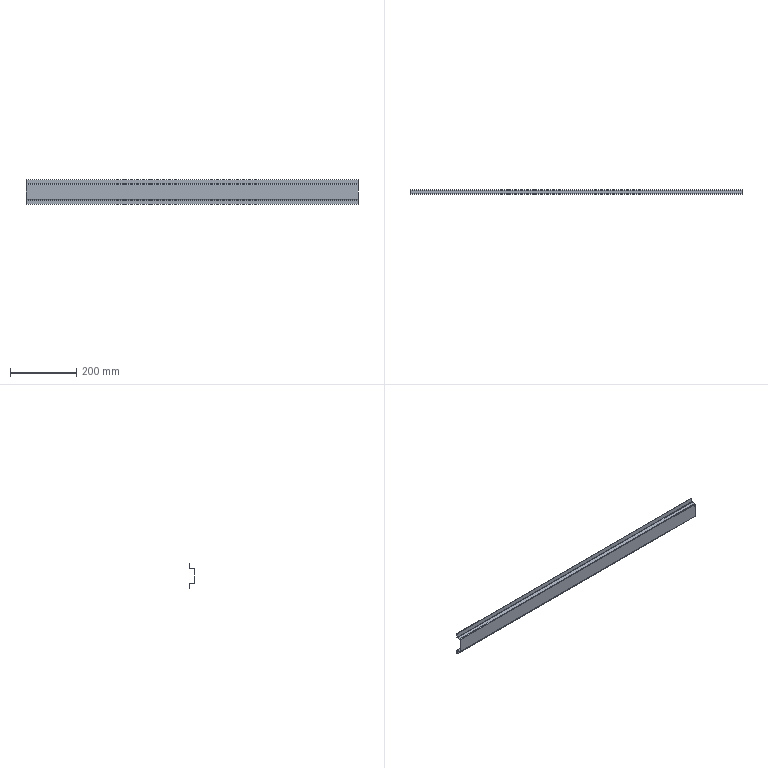Part | SolidWorks | features BaseBody 1 | 1 solid | 22 faces | box 1005 x 14.5 x 75 mm | volume 100376 mm3 | plane 14 | cylinder 8 | commonest cylinder face diameters 1.473 x4 3.473 x4
STEP:
#1=CARTESIAN_POINT('',(502.5,0.,21.763));
#2=VERTEX_POINT('',#1);
#3=CARTESIAN_POINT('',(-502.5,0.,21.763));
#4=VERTEX_POINT('',#3);
#5=CARTESIAN_POINT('',(502.5,0.,21.763));
#6=DIRECTION('',(-1.,0.,0.));
#7=VECTOR('',#6,1000.);
#8=LINE('',#5,#7);
#9=EDGE_CURVE('',#2,#4,#8,.T.);
#10=ORIENTED_EDGE('',*,*,#9,.F.);
#11=CARTESIAN_POINT('',(502.5,0.,-21.763));
#12=VERTEX_POINT('',#11);
#13=CARTESIAN_POINT('',(502.5,0.,22.5));
#14=DIRECTION('',(0.,0.,1.));
#15=VECTOR('',#14,1000.);
#16=LINE('',#13,#15);
#17=EDGE_CURVE('',#12,#2,#16,.T.);
#18=ORIENTED_EDGE('',*,*,#17,.F.);
#19=CARTESIAN_POINT('',(-502.5,0.,-21.763));
#20=VERTEX_POINT('',#19);
#21=CARTESIAN_POINT('',(502.5,0.,-21.763));
#22=DIRECTION('',(1.,0.,0.));
#23=VECTOR('',#22,1000.);
#24=LINE('',#21,#23);
#25=EDGE_CURVE('',#20,#12,#24,.T.);
#26=ORIENTED_EDGE('',*,*,#25,.F.);
#27=CARTESIAN_POINT('',(-502.5,0.,22.5));
#28=DIRECTION('',(0.,0.,-1.));
#29=VECTOR('',#28,1000.);
#30=LINE('',#27,#29);
#31=EDGE_CURVE('',#4,#20,#30,.T.);
#32=ORIENTED_EDGE('',*,*,#31,.F.);
#33=EDGE_LOOP('',(#10,#18,#26,#32));
#34=FACE_OUTER_BOUND('',#33,.T.);
#35=CARTESIAN_POINT('',(502.5,0.,22.5));
#36=DIRECTION('',(0.,-1.,0.));
#37=DIRECTION('',(0.,0.,-1.));
#38=AXIS2_PLACEMENT_3D('',#35,#36,#37);
#39=PLANE('',#38);
#40=ADVANCED_FACE('',(#34),#39,.F.);
#41=CARTESIAN_POINT('',(-502.5,-1.,-21.763));
#42=VERTEX_POINT('',#41);
#43=CARTESIAN_POINT('',(-502.5,-1.,21.763));
#44=VERTEX_POINT('',#43);
#45=CARTESIAN_POINT('',(-502.5,-1.,-23.5));
#46=DIRECTION('',(0.,0.,1.));
#47=VECTOR('',#46,1000.);
#48=LINE('',#45,#47);
#49=EDGE_CURVE('',#42,#44,#48,.T.);
#50=ORIENTED_EDGE('',*,*,#49,.T.);
#51=CARTESIAN_POINT('',(-502.5,0.7366,23.5));
#52=VERTEX_POINT('',#51);
#53=CARTESIAN_POINT('',(-502.5,0.7366,21.763));
#54=DIRECTION('',(1.,0.,0.));
#55=DIRECTION('',(0.,0.,1.));
#56=AXIS2_PLACEMENT_3D('',#53,#54,#55);
#57=CIRCLE('',#56,1.737);
#58=EDGE_CURVE('',#52,#44,#57,.T.);
#59=ORIENTED_EDGE('',*,*,#58,.F.);
#60=CARTESIAN_POINT('',(-502.5,11.763,23.5));
#61=VERTEX_POINT('',#60);
#62=CARTESIAN_POINT('',(-502.5,-1.,23.5));
#63=DIRECTION('',(0.,1.,0.));
#64=VECTOR('',#63,1000.);
#65=LINE('',#62,#64);
#66=EDGE_CURVE('',#52,#61,#65,.T.);
#67=ORIENTED_EDGE('',*,*,#66,.T.);
#68=CARTESIAN_POINT('',(-502.5,12.5,24.237));
#69=VERTEX_POINT('',#68);
#70=CARTESIAN_POINT('',(-502.5,11.763,24.237));
#71=DIRECTION('',(1.,0.,0.));
#72=DIRECTION('',(0.,0.,1.));
#73=AXIS2_PLACEMENT_3D('',#70,#71,#72);
#74=CIRCLE('',#73,0.7366);
#75=EDGE_CURVE('',#61,#69,#74,.T.);
#76=ORIENTED_EDGE('',*,*,#75,.T.);
#77=CARTESIAN_POINT('',(-502.5,12.5,37.5));
#78=VERTEX_POINT('',#77);
#79=CARTESIAN_POINT('',(-502.5,12.5,23.5));
#80=DIRECTION('',(0.,0.,1.));
#81=VECTOR('',#80,1000.);
#82=LINE('',#79,#81);
#83=EDGE_CURVE('',#69,#78,#82,.T.);
#84=ORIENTED_EDGE('',*,*,#83,.T.);
#85=CARTESIAN_POINT('',(-502.5,13.5,37.5));
#86=VERTEX_POINT('',#85);
#87=CARTESIAN_POINT('',(-502.5,11.763,37.5));
#88=DIRECTION('',(0.,1.,0.));
#89=VECTOR('',#88,1000.);
#90=LINE('',#87,#89);
#91=EDGE_CURVE('',#78,#86,#90,.T.);
#92=ORIENTED_EDGE('',*,*,#91,.T.);
#93=CARTESIAN_POINT('',(-502.5,13.5,24.237));
#94=VERTEX_POINT('',#93);
#95=CARTESIAN_POINT('',(-502.5,13.5,22.5));
#96=DIRECTION('',(0.,0.,-1.));
#97=VECTOR('',#96,1000.);
#98=LINE('',#95,#97);
#99=EDGE_CURVE('',#86,#94,#98,.T.);
#100=ORIENTED_EDGE('',*,*,#99,.T.);
#101=CARTESIAN_POINT('',(-502.5,11.763,22.5));
#102=VERTEX_POINT('',#101);
#103=CARTESIAN_POINT('',(-502.5,11.763,24.237));
#104=DIRECTION('',(1.,0.,0.));
#105=DIRECTION('',(0.,0.,1.));
#106=AXIS2_PLACEMENT_3D('',#103,#104,#105);
#107=CIRCLE('',#106,1.737);
#108=EDGE_CURVE('',#102,#94,#107,.T.);
#109=ORIENTED_EDGE('',*,*,#108,.F.);
#110=CARTESIAN_POINT('',(-502.5,0.7366,22.5));
#111=VERTEX_POINT('',#110);
#112=CARTESIAN_POINT('',(-502.5,0.,22.5));
#113=DIRECTION('',(0.,-1.,0.));
#114=VECTOR('',#113,1000.);
#115=LINE('',#112,#114);
#116=EDGE_CURVE('',#102,#111,#115,.T.);
#117=ORIENTED_EDGE('',*,*,#116,.T.);
#118=CARTESIAN_POINT('',(-502.5,0.7366,21.763));
#119=DIRECTION('',(1.,0.,0.));
#120=DIRECTION('',(0.,0.,1.));
#121=AXIS2_PLACEMENT_3D('',#118,#119,#120);
#122=CIRCLE('',#121,0.7366);
#123=EDGE_CURVE('',#111,#4,#122,.T.);
#124=ORIENTED_EDGE('',*,*,#123,.T.);
#125=ORIENTED_EDGE('',*,*,#31,.T.);
#126=CARTESIAN_POINT('',(-502.5,0.7366,-22.5));
#127=VERTEX_POINT('',#126);
#128=CARTESIAN_POINT('',(-502.5,0.7366,-21.763));
#129=DIRECTION('',(1.,0.,0.));
#130=DIRECTION('',(0.,0.,1.));
#131=AXIS2_PLACEMENT_3D('',#128,#129,#130);
#132=CIRCLE('',#131,0.7366);
#133=EDGE_CURVE('',#20,#127,#132,.T.);
#134=ORIENTED_EDGE('',*,*,#133,.T.);
#135=CARTESIAN_POINT('',(-502.5,11.763,-22.5));
#136=VERTEX_POINT('',#135);
#137=CARTESIAN_POINT('',(-502.5,0.,-22.5));
#138=DIRECTION('',(0.,1.,0.));
#139=VECTOR('',#138,1000.);
#140=LINE('',#137,#139);
#141=EDGE_CURVE('',#127,#136,#140,.T.);
#142=ORIENTED_EDGE('',*,*,#141,.T.);
#143=CARTESIAN_POINT('',(-502.5,13.5,-24.237));
#144=VERTEX_POINT('',#143);
#145=CARTESIAN_POINT('',(-502.5,11.763,-24.237));
#146=DIRECTION('',(1.,0.,0.));
#147=DIRECTION('',(0.,0.,1.));
#148=AXIS2_PLACEMENT_3D('',#145,#146,#147);
#149=CIRCLE('',#148,1.737);
#150=EDGE_CURVE('',#144,#136,#149,.T.);
#151=ORIENTED_EDGE('',*,*,#150,.F.);
#152=CARTESIAN_POINT('',(-502.5,13.5,-37.5));
#153=VERTEX_POINT('',#152);
#154=CARTESIAN_POINT('',(-502.5,13.5,-22.5));
#155=DIRECTION('',(0.,0.,-1.));
#156=VECTOR('',#155,1000.);
#157=LINE('',#154,#156);
#158=EDGE_CURVE('',#144,#153,#157,.T.);
#159=ORIENTED_EDGE('',*,*,#158,.T.);
#160=CARTESIAN_POINT('',(-502.5,12.5,-37.5));
#161=VERTEX_POINT('',#160);
#162=CARTESIAN_POINT('',(-502.5,11.763,-37.5));
#163=DIRECTION('',(0.,1.,0.));
#164=VECTOR('',#163,1000.);
#165=LINE('',#162,#164);
#166=EDGE_CURVE('',#161,#153,#165,.T.);
#167=ORIENTED_EDGE('',*,*,#166,.F.);
#168=CARTESIAN_POINT('',(-502.5,12.5,-24.237));
#169=VERTEX_POINT('',#168);
#170=CARTESIAN_POINT('',(-502.5,12.5,24.237));
#171=DIRECTION('',(0.,0.,-1.));
#172=VECTOR('',#171,1000.);
#173=LINE('',#170,#172);
#174=EDGE_CURVE('',#169,#161,#173,.T.);
#175=ORIENTED_EDGE('',*,*,#174,.F.);
#176=CARTESIAN_POINT('',(-502.5,11.763,-23.5));
#177=VERTEX_POINT('',#176);
#178=CARTESIAN_POINT('',(-502.5,11.763,-24.237));
#179=DIRECTION('',(1.,0.,0.));
#180=DIRECTION('',(0.,0.,1.));
#181=AXIS2_PLACEMENT_3D('',#178,#179,#180);
#182=CIRCLE('',#181,0.7366);
#183=EDGE_CURVE('',#169,#177,#182,.T.);
#184=ORIENTED_EDGE('',*,*,#183,.T.);
#185=CARTESIAN_POINT('',(-502.5,0.7366,-23.5));
#186=VERTEX_POINT('',#185);
#187=CARTESIAN_POINT('',(-502.5,12.5,-23.5));
#188=DIRECTION('',(0.,-1.,0.));
#189=VECTOR('',#188,1000.);
#190=LINE('',#187,#189);
#191=EDGE_CURVE('',#177,#186,#190,.T.);
#192=ORIENTED_EDGE('',*,*,#191,.T.);
#193=CARTESIAN_POINT('',(-502.5,0.7366,-21.763));
#194=DIRECTION('',(1.,0.,0.));
#195=DIRECTION('',(0.,0.,1.));
#196=AXIS2_PLACEMENT_3D('',#193,#194,#195);
#197=CIRCLE('',#196,1.737);
#198=EDGE_CURVE('',#42,#186,#197,.T.);
#199=ORIENTED_EDGE('',*,*,#198,.F.);
#200=EDGE_LOOP('',(#50,#59,#67,#76,#84,#92,#100,#109,#117,#124,#125,#134,#142,#151,#159,#167,#175,#184,#192,#199));
#201=FACE_OUTER_BOUND('',#200,.T.);
#202=CARTESIAN_POINT('',(-502.5,0.7366,-23.5));
#203=DIRECTION('',(-1.,0.,0.));
#204=DIRECTION('',(0.,0.,1.));
#205=AXIS2_PLACEMENT_3D('',#202,#203,#204);
#206=PLANE('',#205);
#207=ADVANCED_FACE('',(#201),#206,.T.);
#208=CARTESIAN_POINT('',(502.5,0.7366,22.5));
#209=VERTEX_POINT('',#208);
#210=CARTESIAN_POINT('',(502.5,0.7366,22.5));
#211=DIRECTION('',(-1.,0.,0.));
#212=VECTOR('',#211,1000.);
#213=LINE('',#210,#212);
#214=EDGE_CURVE('',#209,#111,#213,.T.);
#215=ORIENTED_EDGE('',*,*,#214,.F.);
#216=CARTESIAN_POINT('',(502.5,0.7366,21.763));
#217=DIRECTION('',(-1.,0.,0.));
#218=DIRECTION('',(0.,0.,1.));
#219=AXIS2_PLACEMENT_3D('',#216,#217,#218);
#220=CIRCLE('',#219,0.7366);
#221=EDGE_CURVE('',#2,#209,#220,.T.);
#222=ORIENTED_EDGE('',*,*,#221,.F.);
#223=ORIENTED_EDGE('',*,*,#9,.T.);
#224=ORIENTED_EDGE('',*,*,#123,.F.);
#225=EDGE_LOOP('',(#215,#222,#223,#224));
#226=FACE_OUTER_BOUND('',#225,.T.);
#227=CARTESIAN_POINT('',(502.5,0.7366,21.763));
#228=DIRECTION('',(-1.,0.,0.));
#229=DIRECTION('',(0.,0.,1.));
#230=AXIS2_PLACEMENT_3D('',#227,#228,#229);
#231=CYLINDRICAL_SURFACE('',#230,0.7366);
#232=ADVANCED_FACE('',(#226),#231,.F.);
#233=CARTESIAN_POINT('',(502.5,-1.,21.763));
#234=VERTEX_POINT('',#233);
#235=CARTESIAN_POINT('',(502.5,-1.,-21.763));
#236=VERTEX_POINT('',#235);
#237=CARTESIAN_POINT('',(502.5,-1.,23.5));
#238=DIRECTION('',(0.,0.,-1.));
#239=VECTOR('',#238,1000.);
#240=LINE('',#237,#239);
#241=EDGE_CURVE('',#234,#236,#240,.T.);
#242=ORIENTED_EDGE('',*,*,#241,.T.);
#243=CARTESIAN_POINT('',(502.5,0.7366,-23.5));
#244=VERTEX_POINT('',#243);
#245=CARTESIAN_POINT('',(502.5,0.7366,-21.763));
#246=DIRECTION('',(-1.,0.,0.));
#247=DIRECTION('',(0.,0.,1.));
#248=AXIS2_PLACEMENT_3D('',#245,#246,#247);
#249=CIRCLE('',#248,1.737);
#250=EDGE_CURVE('',#244,#236,#249,.T.);
#251=ORIENTED_EDGE('',*,*,#250,.F.);
#252=CARTESIAN_POINT('',(502.5,11.763,-23.5));
#253=VERTEX_POINT('',#252);
#254=CARTESIAN_POINT('',(502.5,-1.,-23.5));
#255=DIRECTION('',(0.,1.,0.));
#256=VECTOR('',#255,1000.);
#257=LINE('',#254,#256);
#258=EDGE_CURVE('',#244,#253,#257,.T.);
#259=ORIENTED_EDGE('',*,*,#258,.T.);
#260=CARTESIAN_POINT('',(502.5,12.5,-24.237));
#261=VERTEX_POINT('',#260);
#262=CARTESIAN_POINT('',(502.5,11.763,-24.237));
#263=DIRECTION('',(-1.,0.,0.));
#264=DIRECTION('',(0.,0.,1.));
#265=AXIS2_PLACEMENT_3D('',#262,#263,#264);
#266=CIRCLE('',#265,0.7366);
#267=EDGE_CURVE('',#253,#261,#266,.T.);
#268=ORIENTED_EDGE('',*,*,#267,.T.);
#269=CARTESIAN_POINT('',(502.5,12.5,-37.5));
#270=VERTEX_POINT('',#269);
#271=CARTESIAN_POINT('',(502.5,12.5,-23.5));
#272=DIRECTION('',(0.,0.,-1.));
#273=VECTOR('',#272,1000.);
#274=LINE('',#271,#273);
#275=EDGE_CURVE('',#261,#270,#274,.T.);
#276=ORIENTED_EDGE('',*,*,#275,.T.);
#277=CARTESIAN_POINT('',(502.5,13.5,-37.5));
#278=VERTEX_POINT('',#277);
#279=CARTESIAN_POINT('',(502.5,11.763,-37.5));
#280=DIRECTION('',(0.,1.,0.));
#281=VECTOR('',#280,1000.);
#282=LINE('',#279,#281);
#283=EDGE_CURVE('',#270,#278,#282,.T.);
#284=ORIENTED_EDGE('',*,*,#283,.T.);
#285=CARTESIAN_POINT('',(502.5,13.5,-24.237));
#286=VERTEX_POINT('',#285);
#287=CARTESIAN_POINT('',(502.5,13.5,-22.5));
#288=DIRECTION('',(0.,0.,1.));
#289=VECTOR('',#288,1000.);
#290=LINE('',#287,#289);
#291=EDGE_CURVE('',#278,#286,#290,.T.);
#292=ORIENTED_EDGE('',*,*,#291,.T.);
#293=CARTESIAN_POINT('',(502.5,11.763,-22.5));
#294=VERTEX_POINT('',#293);
#295=CARTESIAN_POINT('',(502.5,11.763,-24.237));
#296=DIRECTION('',(-1.,0.,0.));
#297=DIRECTION('',(0.,0.,1.));
#298=AXIS2_PLACEMENT_3D('',#295,#296,#297);
#299=CIRCLE('',#298,1.737);
#300=EDGE_CURVE('',#294,#286,#299,.T.);
#301=ORIENTED_EDGE('',*,*,#300,.F.);
#302=CARTESIAN_POINT('',(502.5,0.7366,-22.5));
#303=VERTEX_POINT('',#302);
#304=CARTESIAN_POINT('',(502.5,0.,-22.5));
#305=DIRECTION('',(0.,-1.,0.));
#306=VECTOR('',#305,1000.);
#307=LINE('',#304,#306);
#308=EDGE_CURVE('',#294,#303,#307,.T.);
#309=ORIENTED_EDGE('',*,*,#308,.T.);
#310=CARTESIAN_POINT('',(502.5,0.7366,-21.763));
#311=DIRECTION('',(-1.,0.,0.));
#312=DIRECTION('',(0.,0.,1.));
#313=AXIS2_PLACEMENT_3D('',#310,#311,#312);
#314=CIRCLE('',#313,0.7366);
#315=EDGE_CURVE('',#303,#12,#314,.T.);
#316=ORIENTED_EDGE('',*,*,#315,.T.);
#317=ORIENTED_EDGE('',*,*,#17,.T.);
#318=ORIENTED_EDGE('',*,*,#221,.T.);
#319=CARTESIAN_POINT('',(502.5,11.763,22.5));
#320=VERTEX_POINT('',#319);
#321=CARTESIAN_POINT('',(502.5,0.,22.5));
#322=DIRECTION('',(0.,1.,0.));
#323=VECTOR('',#322,1000.);
#324=LINE('',#321,#323);
#325=EDGE_CURVE('',#209,#320,#324,.T.);
#326=ORIENTED_EDGE('',*,*,#325,.T.);
#327=CARTESIAN_POINT('',(502.5,13.5,24.237));
#328=VERTEX_POINT('',#327);
#329=CARTESIAN_POINT('',(502.5,11.763,24.237));
#330=DIRECTION('',(-1.,0.,0.));
#331=DIRECTION('',(0.,0.,1.));
#332=AXIS2_PLACEMENT_3D('',#329,#330,#331);
#333=CIRCLE('',#332,1.737);
#334=EDGE_CURVE('',#328,#320,#333,.T.);
#335=ORIENTED_EDGE('',*,*,#334,.F.);
#336=CARTESIAN_POINT('',(502.5,13.5,37.5));
#337=VERTEX_POINT('',#336);
#338=CARTESIAN_POINT('',(502.5,13.5,22.5));
#339=DIRECTION('',(0.,0.,1.));
#340=VECTOR('',#339,1000.);
#341=LINE('',#338,#340);
#342=EDGE_CURVE('',#328,#337,#341,.T.);
#343=ORIENTED_EDGE('',*,*,#342,.T.);
#344=CARTESIAN_POINT('',(502.5,12.5,37.5));
#345=VERTEX_POINT('',#344);
#346=CARTESIAN_POINT('',(502.5,12.5,37.5));
#347=DIRECTION('',(0.,1.,0.));
#348=VECTOR('',#347,1000.);
#349=LINE('',#346,#348);
#350=EDGE_CURVE('',#345,#337,#349,.T.);
#351=ORIENTED_EDGE('',*,*,#350,.F.);
#352=CARTESIAN_POINT('',(502.5,12.5,24.237));
#353=VERTEX_POINT('',#352);
#354=CARTESIAN_POINT('',(502.5,12.5,24.237));
#355=DIRECTION('',(0.,0.,-1.));
#356=VECTOR('',#355,1000.);
#357=LINE('',#354,#356);
#358=EDGE_CURVE('',#345,#353,#357,.T.);
#359=ORIENTED_EDGE('',*,*,#358,.T.);
#360=CARTESIAN_POINT('',(502.5,11.763,23.5));
#361=VERTEX_POINT('',#360);
#362=CARTESIAN_POINT('',(502.5,11.763,24.237));
#363=DIRECTION('',(-1.,0.,0.));
#364=DIRECTION('',(0.,0.,1.));
#365=AXIS2_PLACEMENT_3D('',#362,#363,#364);
#366=CIRCLE('',#365,0.7366);
#367=EDGE_CURVE('',#353,#361,#366,.T.);
#368=ORIENTED_EDGE('',*,*,#367,.T.);
#369=CARTESIAN_POINT('',(502.5,0.7366,23.5));
#370=VERTEX_POINT('',#369);
#371=CARTESIAN_POINT('',(502.5,12.5,23.5));
#372=DIRECTION('',(0.,-1.,0.));
#373=VECTOR('',#372,1000.);
#374=LINE('',#371,#373);
#375=EDGE_CURVE('',#361,#370,#374,.T.);
#376=ORIENTED_EDGE('',*,*,#375,.T.);
#377=CARTESIAN_POINT('',(502.5,0.7366,21.763));
#378=DIRECTION('',(-1.,0.,0.));
#379=DIRECTION('',(0.,0.,1.));
#380=AXIS2_PLACEMENT_3D('',#377,#378,#379);
#381=CIRCLE('',#380,1.737);
#382=EDGE_CURVE('',#234,#370,#381,.T.);
#383=ORIENTED_EDGE('',*,*,#382,.F.);
#384=EDGE_LOOP('',(#242,#251,#259,#268,#276,#284,#292,#301,#309,#316,#317,#318,#326,#335,#343,#351,#359,#368,#376,#383));
#385=FACE_OUTER_BOUND('',#384,.T.);
#386=CARTESIAN_POINT('',(502.5,0.7366,23.5));
#387=DIRECTION('',(1.,0.,0.));
#388=DIRECTION('',(0.,0.,-1.));
#389=AXIS2_PLACEMENT_3D('',#386,#387,#388);
#390=PLANE('',#389);
#391=ADVANCED_FACE('',(#385),#390,.T.);
#392=ORIENTED_EDGE('',*,*,#25,.T.);
#393=ORIENTED_EDGE('',*,*,#315,.F.);
#394=CARTESIAN_POINT('',(502.5,0.7366,-22.5));
#395=DIRECTION('',(1.,0.,0.));
#396=VECTOR('',#395,1000.);
#397=LINE('',#394,#396);
#398=EDGE_CURVE('',#127,#303,#397,.T.);
#399=ORIENTED_EDGE('',*,*,#398,.F.);
#400=ORIENTED_EDGE('',*,*,#133,.F.);
#401=EDGE_LOOP('',(#392,#393,#399,#400));
#402=FACE_OUTER_BOUND('',#401,.T.);
#403=CARTESIAN_POINT('',(502.5,0.7366,-21.763));
#404=DIRECTION('',(-1.,0.,0.));
#405=DIRECTION('',(0.,0.,1.));
#406=AXIS2_PLACEMENT_3D('',#403,#404,#405);
#407=CYLINDRICAL_SURFACE('',#406,0.7366);
#408=ADVANCED_FACE('',(#402),#407,.F.);
#409=ORIENTED_EDGE('',*,*,#241,.F.);
#410=CARTESIAN_POINT('',(502.5,-1.,21.763));
#411=DIRECTION('',(-1.,0.,0.));
#412=VECTOR('',#411,1000.);
#413=LINE('',#410,#412);
#414=EDGE_CURVE('',#234,#44,#413,.T.);
#415=ORIENTED_EDGE('',*,*,#414,.T.);
#416=ORIENTED_EDGE('',*,*,#49,.F.);
#417=CARTESIAN_POINT('',(502.5,-1.,-21.763));
#418=DIRECTION('',(1.,0.,0.));
#419=VECTOR('',#418,1000.);
#420=LINE('',#417,#419);
#421=EDGE_CURVE('',#42,#236,#420,.T.);
#422=ORIENTED_EDGE('',*,*,#421,.T.);
#423=EDGE_LOOP('',(#409,#415,#416,#422));
#424=FACE_OUTER_BOUND('',#423,.T.);
#425=CARTESIAN_POINT('',(502.5,-1.,22.5));
#426=DIRECTION('',(0.,-1.,0.));
#427=DIRECTION('',(0.,0.,-1.));
#428=AXIS2_PLACEMENT_3D('',#425,#426,#427);
#429=PLANE('',#428);
#430=ADVANCED_FACE('',(#424),#429,.T.);
#431=CARTESIAN_POINT('',(502.5,11.763,22.5));
#432=DIRECTION('',(-1.,0.,0.));
#433=VECTOR('',#432,1000.);
#434=LINE('',#431,#433);
#435=EDGE_CURVE('',#320,#102,#434,.T.);
#436=ORIENTED_EDGE('',*,*,#435,.F.);
#437=ORIENTED_EDGE('',*,*,#325,.F.);
#438=ORIENTED_EDGE('',*,*,#214,.T.);
#439=ORIENTED_EDGE('',*,*,#116,.F.);
#440=EDGE_LOOP('',(#436,#437,#438,#439));
#441=FACE_OUTER_BOUND('',#440,.T.);
#442=CARTESIAN_POINT('',(502.5,0.,22.5));
#443=DIRECTION('',(0.,0.,1.));
#444=DIRECTION('',(1.,0.,0.));
#445=AXIS2_PLACEMENT_3D('',#442,#443,#444);
#446=PLANE('',#445);
#447=ADVANCED_FACE('',(#441),#446,.F.);
#448=ORIENTED_EDGE('',*,*,#398,.T.);
#449=ORIENTED_EDGE('',*,*,#308,.F.);
#450=CARTESIAN_POINT('',(502.5,11.763,-22.5));
#451=DIRECTION('',(1.,0.,0.));
#452=VECTOR('',#451,1000.);
#453=LINE('',#450,#452);
#454=EDGE_CURVE('',#136,#294,#453,.T.);
#455=ORIENTED_EDGE('',*,*,#454,.F.);
#456=ORIENTED_EDGE('',*,*,#141,.F.);
#457=EDGE_LOOP('',(#448,#449,#455,#456));
#458=FACE_OUTER_BOUND('',#457,.T.);
#459=CARTESIAN_POINT('',(502.5,0.,-22.5));
#460=DIRECTION('',(0.,0.,-1.));
#461=DIRECTION('',(-1.,0.,0.));
#462=AXIS2_PLACEMENT_3D('',#459,#460,#461);
#463=PLANE('',#462);
#464=ADVANCED_FACE('',(#458),#463,.F.);
#465=ORIENTED_EDGE('',*,*,#382,.T.);
#466=CARTESIAN_POINT('',(502.5,0.7366,23.5));
#467=DIRECTION('',(-1.,0.,0.));
#468=VECTOR('',#467,1000.);
#469=LINE('',#466,#468);
#470=EDGE_CURVE('',#370,#52,#469,.T.);
#471=ORIENTED_EDGE('',*,*,#470,.T.);
#472=ORIENTED_EDGE('',*,*,#58,.T.);
#473=ORIENTED_EDGE('',*,*,#414,.F.);
#474=EDGE_LOOP('',(#465,#471,#472,#473));
#475=FACE_OUTER_BOUND('',#474,.T.);
#476=CARTESIAN_POINT('',(502.5,0.7366,21.763));
#477=DIRECTION('',(-1.,0.,0.));
#478=DIRECTION('',(0.,0.,1.));
#479=AXIS2_PLACEMENT_3D('',#476,#477,#478);
#480=CYLINDRICAL_SURFACE('',#479,1.737);
#481=ADVANCED_FACE('',(#475),#480,.T.);
#482=ORIENTED_EDGE('',*,*,#250,.T.);
#483=ORIENTED_EDGE('',*,*,#421,.F.);
#484=ORIENTED_EDGE('',*,*,#198,.T.);
#485=CARTESIAN_POINT('',(502.5,0.7366,-23.5));
#486=DIRECTION('',(1.,0.,0.));
#487=VECTOR('',#486,1000.);
#488=LINE('',#485,#487);
#489=EDGE_CURVE('',#186,#244,#488,.T.);
#490=ORIENTED_EDGE('',*,*,#489,.T.);
#491=EDGE_LOOP('',(#482,#483,#484,#490));
#492=FACE_OUTER_BOUND('',#491,.T.);
#493=CARTESIAN_POINT('',(502.5,0.7366,-21.763));
#494=DIRECTION('',(-1.,0.,0.));
#495=DIRECTION('',(0.,0.,1.));
#496=AXIS2_PLACEMENT_3D('',#493,#494,#495);
#497=CYLINDRICAL_SURFACE('',#496,1.737);
#498=ADVANCED_FACE('',(#492),#497,.T.);
#499=ORIENTED_EDGE('',*,*,#334,.T.);
#500=ORIENTED_EDGE('',*,*,#435,.T.);
#501=ORIENTED_EDGE('',*,*,#108,.T.);
#502=CARTESIAN_POINT('',(502.5,13.5,24.237));
#503=DIRECTION('',(1.,0.,0.));
#504=VECTOR('',#503,1000.);
#505=LINE('',#502,#504);
#506=EDGE_CURVE('',#94,#328,#505,.T.);
#507=ORIENTED_EDGE('',*,*,#506,.T.);
#508=EDGE_LOOP('',(#499,#500,#501,#507));
#509=FACE_OUTER_BOUND('',#508,.T.);
#510=CARTESIAN_POINT('',(502.5,11.763,24.237));
#511=DIRECTION('',(-1.,0.,0.));
#512=DIRECTION('',(0.,0.,1.));
#513=AXIS2_PLACEMENT_3D('',#510,#511,#512);
#514=CYLINDRICAL_SURFACE('',#513,1.737);
#515=ADVANCED_FACE('',(#509),#514,.T.);
#516=ORIENTED_EDGE('',*,*,#300,.T.);
#517=CARTESIAN_POINT('',(502.5,13.5,-24.237));
#518=DIRECTION('',(-1.,0.,0.));
#519=VECTOR('',#518,1000.);
#520=LINE('',#517,#519);
#521=EDGE_CURVE('',#286,#144,#520,.T.);
#522=ORIENTED_EDGE('',*,*,#521,.T.);
#523=ORIENTED_EDGE('',*,*,#150,.T.);
#524=ORIENTED_EDGE('',*,*,#454,.T.);
#525=EDGE_LOOP('',(#516,#522,#523,#524));
#526=FACE_OUTER_BOUND('',#525,.T.);
#527=CARTESIAN_POINT('',(502.5,11.763,-24.237));
#528=DIRECTION('',(-1.,0.,0.));
#529=DIRECTION('',(0.,0.,1.));
#530=AXIS2_PLACEMENT_3D('',#527,#528,#529);
#531=CYLINDRICAL_SURFACE('',#530,1.737);
#532=ADVANCED_FACE('',(#526),#531,.T.);
#533=ORIENTED_EDGE('',*,*,#375,.F.);
#534=CARTESIAN_POINT('',(502.5,11.763,23.5));
#535=DIRECTION('',(-1.,0.,0.));
#536=VECTOR('',#535,1000.);
#537=LINE('',#534,#536);
#538=EDGE_CURVE('',#361,#61,#537,.T.);
#539=ORIENTED_EDGE('',*,*,#538,.T.);
#540=ORIENTED_EDGE('',*,*,#66,.F.);
#541=ORIENTED_EDGE('',*,*,#470,.F.);
#542=EDGE_LOOP('',(#533,#539,#540,#541));
#543=FACE_OUTER_BOUND('',#542,.T.);
#544=CARTESIAN_POINT('',(502.5,0.,23.5));
#545=DIRECTION('',(0.,0.,1.));
#546=DIRECTION('',(1.,0.,0.));
#547=AXIS2_PLACEMENT_3D('',#544,#545,#546);
#548=PLANE('',#547);
#549=ADVANCED_FACE('',(#543),#548,.T.);
#550=ORIENTED_EDGE('',*,*,#258,.F.);
#551=ORIENTED_EDGE('',*,*,#489,.F.);
#552=ORIENTED_EDGE('',*,*,#191,.F.);
#553=CARTESIAN_POINT('',(502.5,11.763,-23.5));
#554=DIRECTION('',(1.,0.,0.));
#555=VECTOR('',#554,1000.);
#556=LINE('',#553,#555);
#557=EDGE_CURVE('',#177,#253,#556,.T.);
#558=ORIENTED_EDGE('',*,*,#557,.T.);
#559=EDGE_LOOP('',(#550,#551,#552,#558));
#560=FACE_OUTER_BOUND('',#559,.T.);
#561=CARTESIAN_POINT('',(502.5,0.,-23.5));
#562=DIRECTION('',(0.,0.,-1.));
#563=DIRECTION('',(-1.,0.,0.));
#564=AXIS2_PLACEMENT_3D('',#561,#562,#563);
#565=PLANE('',#564);
#566=ADVANCED_FACE('',(#560),#565,.T.);
#567=CARTESIAN_POINT('',(502.5,13.5,37.5));
#568=DIRECTION('',(-1.,0.,0.));
#569=VECTOR('',#568,1000.);
#570=LINE('',#567,#569);
#571=EDGE_CURVE('',#337,#86,#570,.T.);
#572=ORIENTED_EDGE('',*,*,#571,.F.);
#573=ORIENTED_EDGE('',*,*,#342,.F.);
#574=ORIENTED_EDGE('',*,*,#506,.F.);
#575=ORIENTED_EDGE('',*,*,#99,.F.);
#576=EDGE_LOOP('',(#572,#573,#574,#575));
#577=FACE_OUTER_BOUND('',#576,.T.);
#578=CARTESIAN_POINT('',(502.5,13.5,22.5));
#579=DIRECTION('',(0.,-1.,0.));
#580=DIRECTION('',(0.,0.,-1.));
#581=AXIS2_PLACEMENT_3D('',#578,#579,#580);
#582=PLANE('',#581);
#583=ADVANCED_FACE('',(#577),#582,.F.);
#584=ORIENTED_EDGE('',*,*,#521,.F.);
#585=ORIENTED_EDGE('',*,*,#291,.F.);
#586=CARTESIAN_POINT('',(502.5,13.5,-37.5));
#587=DIRECTION('',(1.,0.,0.));
#588=VECTOR('',#587,1000.);
#589=LINE('',#586,#588);
#590=EDGE_CURVE('',#153,#278,#589,.T.);
#591=ORIENTED_EDGE('',*,*,#590,.F.);
#592=ORIENTED_EDGE('',*,*,#158,.F.);
#593=EDGE_LOOP('',(#584,#585,#591,#592));
#594=FACE_OUTER_BOUND('',#593,.T.);
#595=CARTESIAN_POINT('',(502.5,13.5,-22.5));
#596=DIRECTION('',(0.,-1.,0.));
#597=DIRECTION('',(0.,0.,-1.));
#598=AXIS2_PLACEMENT_3D('',#595,#596,#597);
#599=PLANE('',#598);
#600=ADVANCED_FACE('',(#594),#599,.F.);
#601=ORIENTED_EDGE('',*,*,#538,.F.);
#602=ORIENTED_EDGE('',*,*,#367,.F.);
#603=CARTESIAN_POINT('',(502.5,12.5,24.237));
#604=DIRECTION('',(1.,0.,0.));
#605=VECTOR('',#604,1000.);
#606=LINE('',#603,#605);
#607=EDGE_CURVE('',#69,#353,#606,.T.);
#608=ORIENTED_EDGE('',*,*,#607,.F.);
#609=ORIENTED_EDGE('',*,*,#75,.F.);
#610=EDGE_LOOP('',(#601,#602,#608,#609));
#611=FACE_OUTER_BOUND('',#610,.T.);
#612=CARTESIAN_POINT('',(502.5,11.763,24.237));
#613=DIRECTION('',(-1.,0.,0.));
#614=DIRECTION('',(0.,0.,1.));
#615=AXIS2_PLACEMENT_3D('',#612,#613,#614);
#616=CYLINDRICAL_SURFACE('',#615,0.7366);
#617=ADVANCED_FACE('',(#611),#616,.F.);
#618=CARTESIAN_POINT('',(502.5,12.5,-24.237));
#619=DIRECTION('',(-1.,0.,0.));
#620=VECTOR('',#619,1000.);
#621=LINE('',#618,#620);
#622=EDGE_CURVE('',#261,#169,#621,.T.);
#623=ORIENTED_EDGE('',*,*,#622,.F.);
#624=ORIENTED_EDGE('',*,*,#267,.F.);
#625=ORIENTED_EDGE('',*,*,#557,.F.);
#626=ORIENTED_EDGE('',*,*,#183,.F.);
#627=EDGE_LOOP('',(#623,#624,#625,#626));
#628=FACE_OUTER_BOUND('',#627,.T.);
#629=CARTESIAN_POINT('',(502.5,11.763,-24.237));
#630=DIRECTION('',(-1.,0.,0.));
#631=DIRECTION('',(0.,0.,1.));
#632=AXIS2_PLACEMENT_3D('',#629,#630,#631);
#633=CYLINDRICAL_SURFACE('',#632,0.7366);
#634=ADVANCED_FACE('',(#628),#633,.F.);
#635=ORIENTED_EDGE('',*,*,#350,.T.);
#636=ORIENTED_EDGE('',*,*,#571,.T.);
#637=ORIENTED_EDGE('',*,*,#91,.F.);
#638=CARTESIAN_POINT('',(502.5,12.5,37.5));
#639=DIRECTION('',(1.,0.,0.));
#640=VECTOR('',#639,1000.);
#641=LINE('',#638,#640);
#642=EDGE_CURVE('',#78,#345,#641,.T.);
#643=ORIENTED_EDGE('',*,*,#642,.T.);
#644=EDGE_LOOP('',(#635,#636,#637,#643));
#645=FACE_OUTER_BOUND('',#644,.T.);
#646=CARTESIAN_POINT('',(502.5,12.5,37.5));
#647=DIRECTION('',(0.,0.,1.));
#648=DIRECTION('',(1.,0.,0.));
#649=AXIS2_PLACEMENT_3D('',#646,#647,#648);
#650=PLANE('',#649);
#651=ADVANCED_FACE('',(#645),#650,.T.);
#652=ORIENTED_EDGE('',*,*,#283,.F.);
#653=CARTESIAN_POINT('',(502.5,12.5,-37.5));
#654=DIRECTION('',(-1.,0.,0.));
#655=VECTOR('',#654,1000.);
#656=LINE('',#653,#655);
#657=EDGE_CURVE('',#270,#161,#656,.T.);
#658=ORIENTED_EDGE('',*,*,#657,.T.);
#659=ORIENTED_EDGE('',*,*,#166,.T.);
#660=ORIENTED_EDGE('',*,*,#590,.T.);
#661=EDGE_LOOP('',(#652,#658,#659,#660));
#662=FACE_OUTER_BOUND('',#661,.T.);
#663=CARTESIAN_POINT('',(502.5,13.5,-37.5));
#664=DIRECTION('',(0.,0.,-1.));
#665=DIRECTION('',(-1.,0.,0.));
#666=AXIS2_PLACEMENT_3D('',#663,#664,#665);
#667=PLANE('',#666);
#668=ADVANCED_FACE('',(#662),#667,.T.);
#669=ORIENTED_EDGE('',*,*,#358,.F.);
#670=ORIENTED_EDGE('',*,*,#642,.F.);
#671=ORIENTED_EDGE('',*,*,#83,.F.);
#672=ORIENTED_EDGE('',*,*,#607,.T.);
#673=EDGE_LOOP('',(#669,#670,#671,#672));
#674=FACE_OUTER_BOUND('',#673,.T.);
#675=CARTESIAN_POINT('',(502.5,12.5,22.5));
#676=DIRECTION('',(0.,-1.,0.));
#677=DIRECTION('',(0.,0.,-1.));
#678=AXIS2_PLACEMENT_3D('',#675,#676,#677);
#679=PLANE('',#678);
#680=ADVANCED_FACE('',(#674),#679,.T.);
#681=ORIENTED_EDGE('',*,*,#275,.F.);
#682=ORIENTED_EDGE('',*,*,#622,.T.);
#683=ORIENTED_EDGE('',*,*,#174,.T.);
#684=ORIENTED_EDGE('',*,*,#657,.F.);
#685=EDGE_LOOP('',(#681,#682,#683,#684));
#686=FACE_OUTER_BOUND('',#685,.T.);
#687=CARTESIAN_POINT('',(502.5,12.5,-22.5));
#688=DIRECTION('',(0.,-1.,0.));
#689=DIRECTION('',(0.,0.,-1.));
#690=AXIS2_PLACEMENT_3D('',#687,#688,#689);
#691=PLANE('',#690);
#692=ADVANCED_FACE('',(#686),#691,.T.);
#693=CLOSED_SHELL('',(#40,#207,#232,#391,#408,#430,#447,#464,#481,#498,#515,#532,#549,#566,#583,#600,#617,#634,#651,#668,#680,#692));
#694=MANIFOLD_SOLID_BREP('',#693);
#695=CARTESIAN_POINT('',(0.,0.,0.));
#696=DIRECTION('',(0.,0.,1.));
#697=DIRECTION('',(1.,0.,0.));
#698=AXIS2_PLACEMENT_3D('',#695,#696,#697);
#699=(LENGTH_UNIT()NAMED_UNIT(*)SI_UNIT(.MILLI.,.METRE.));
#700=UNCERTAINTY_MEASURE_WITH_UNIT(LENGTH_MEASURE(0.00001),#699,'','');
#701=(NAMED_UNIT(*)PLANE_ANGLE_UNIT()SI_UNIT($,.RADIAN.));
#702=(NAMED_UNIT(*)SI_UNIT($,.STERADIAN.)SOLID_ANGLE_UNIT());
#703=(GEOMETRIC_REPRESENTATION_CONTEXT(3)GLOBAL_UNCERTAINTY_ASSIGNED_CONTEXT((#700))GLOBAL_UNIT_ASSIGNED_CONTEXT((#699,#701,#702))REPRESENTATION_CONTEXT('',''));
#704=ADVANCED_BREP_SHAPE_REPRESENTATION('',(#694,#698),#703);